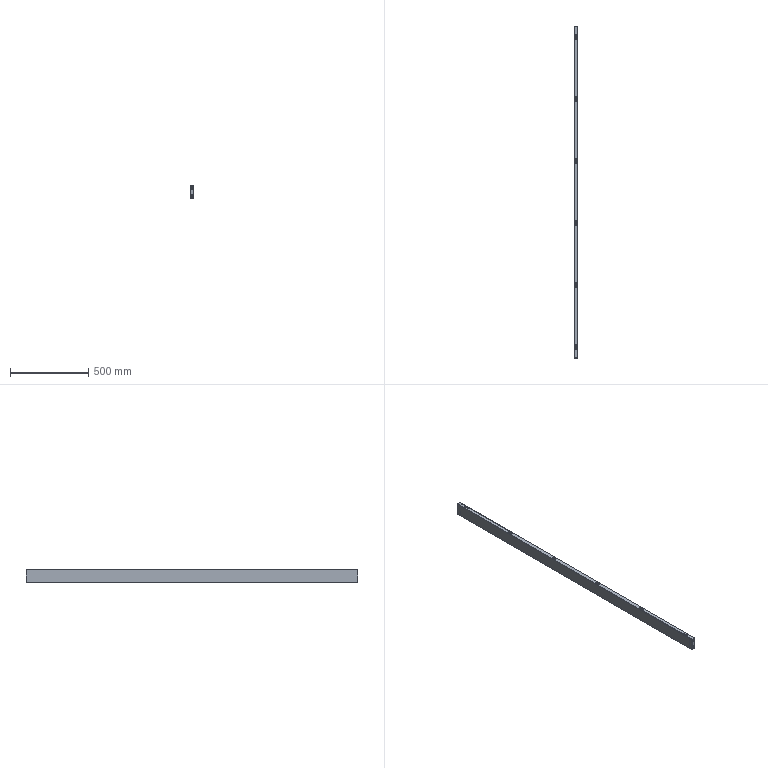Part | SolidWorks | features MirrorCompFeat 1, ReferencePattern 1 | 3 solids | 180 faces | box 25 x 2116 x 80 mm | volume 386202 mm3 | plane 102 | cylinder 78 | commonest cylinder face diameters 6.2 x28 9 x18 10 x12 3.4 x10 0.4 x6 1 x4